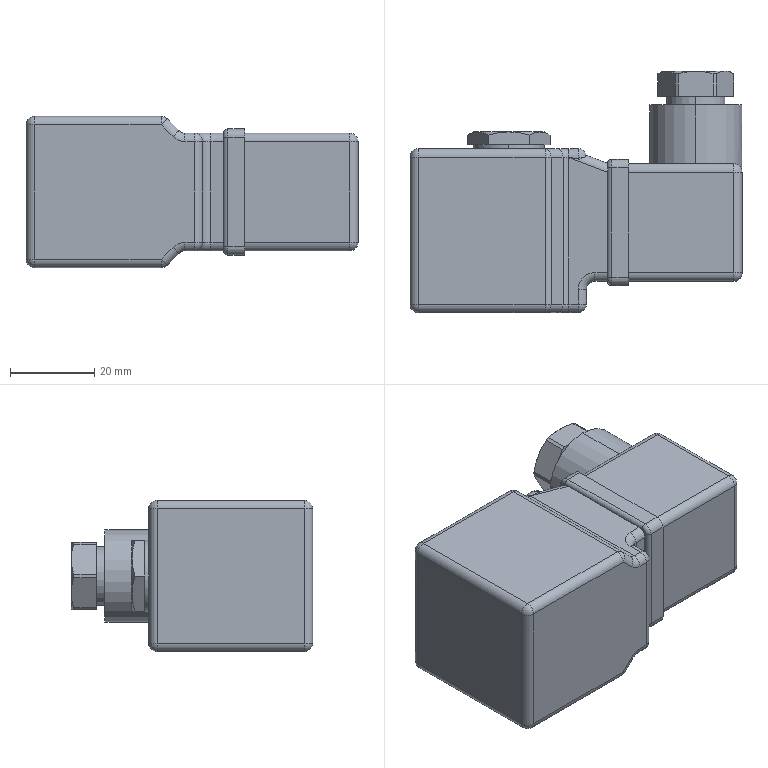Part | SolidWorks | features Fillet 5, Cut 4, Boss 3, Revolution 2, Extrusion 1 | 1 solid | 151 faces | box 79 x 57.43 x 36 mm | volume 93885 mm3 | cylinder 60 | plane 47 | sphere 18 | cone 12 | torus 10 | spline 4 | commonest cylinder face diameters 4 x42 2 x6 18 x6 14 x2 17 x2 22 x2